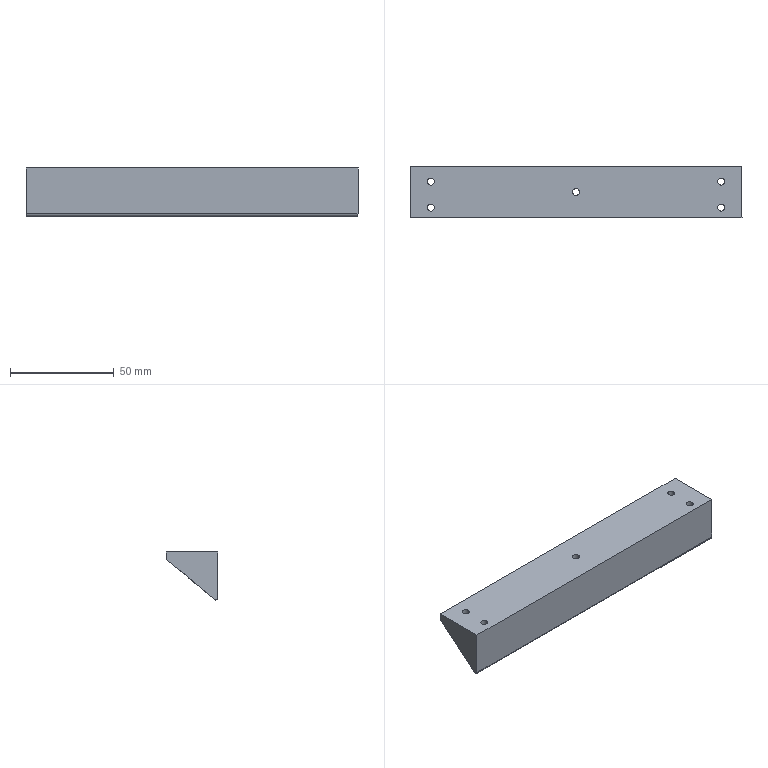Part | SolidWorks | features BaseBody 1, DelFace 1 | 1 solid | 19 faces | box 160 x 25 x 23.134 mm | volume 54327 mm3 | cylinder 13 | plane 6 | commonest cylinder face diameters 3.4 x10 2 x3
STEP:
#1=CARTESIAN_POINT('',(-731.43,686.87,479.692));
#2=VERTEX_POINT('',#1);
#3=CARTESIAN_POINT('',(-734.83,686.87,479.692));
#4=VERTEX_POINT('',#3);
#5=CARTESIAN_POINT('',(-731.43,686.87,479.692));
#6=CARTESIAN_POINT('',(-731.43,690.27,482.545));
#7=CARTESIAN_POINT('',(-734.83,690.27,482.545));
#8=CARTESIAN_POINT('',(-734.83,686.87,479.692));
#9=(BOUNDED_CURVE()B_SPLINE_CURVE(3,(#5,#6,#7,#8),.UNSPECIFIED.,.F.,.F.)B_SPLINE_CURVE_WITH_KNOTS((4,4),(4.712,7.854),.UNSPECIFIED.)CURVE()GEOMETRIC_REPRESENTATION_ITEM()RATIONAL_B_SPLINE_CURVE((1.,0.3333,0.3333,1.))REPRESENTATION_ITEM(''));
#10=EDGE_CURVE('',#2,#4,#9,.T.);
#11=ORIENTED_EDGE('',*,*,#10,.F.);
#12=CARTESIAN_POINT('',(-731.43,686.87,493.482));
#13=VERTEX_POINT('',#12);
#14=CARTESIAN_POINT('',(-731.43,686.87,493.482));
#15=DIRECTION('',(0.,0.,1.));
#16=VECTOR('',#15,1000.);
#17=LINE('',#14,#16);
#18=EDGE_CURVE('',#2,#13,#17,.T.);
#19=ORIENTED_EDGE('',*,*,#18,.T.);
#20=CARTESIAN_POINT('',(-734.83,686.87,493.482));
#21=VERTEX_POINT('',#20);
#22=CARTESIAN_POINT('',(-733.13,686.87,493.482));
#23=DIRECTION('',(0.,0.,1.));
#24=DIRECTION('',(-0.000001544,1.,0.));
#25=AXIS2_PLACEMENT_3D('',#22,#23,#24);
#26=CIRCLE('',#25,1.7);
#27=EDGE_CURVE('',#13,#21,#26,.T.);
#28=ORIENTED_EDGE('',*,*,#27,.T.);
#29=CARTESIAN_POINT('',(-734.83,686.87,493.482));
#30=DIRECTION('',(0.,0.,1.));
#31=VECTOR('',#30,1000.);
#32=LINE('',#29,#31);
#33=EDGE_CURVE('',#4,#21,#32,.T.);
#34=ORIENTED_EDGE('',*,*,#33,.F.);
#35=EDGE_LOOP('',(#11,#19,#28,#34));
#36=FACE_OUTER_BOUND('',#35,.T.);
#37=CARTESIAN_POINT('',(-733.13,686.87,493.482));
#38=DIRECTION('',(0.,0.,1.));
#39=DIRECTION('',(-1.,-0.000001544,0.));
#40=AXIS2_PLACEMENT_3D('',#37,#38,#39);
#41=CYLINDRICAL_SURFACE('',#40,1.7);
#42=ADVANCED_FACE('',(#36),#41,.F.);
#43=CARTESIAN_POINT('',(-661.43,691.87,483.888));
#44=VERTEX_POINT('',#43);
#45=CARTESIAN_POINT('',(-664.83,691.87,483.888));
#46=VERTEX_POINT('',#45);
#47=CARTESIAN_POINT('',(-661.43,691.87,483.888));
#48=CARTESIAN_POINT('',(-661.43,695.27,486.741));
#49=CARTESIAN_POINT('',(-664.83,695.27,486.741));
#50=CARTESIAN_POINT('',(-664.83,691.87,483.888));
#51=(BOUNDED_CURVE()B_SPLINE_CURVE(3,(#47,#48,#49,#50),.UNSPECIFIED.,.F.,.F.)B_SPLINE_CURVE_WITH_KNOTS((4,4),(4.712,7.854),.UNSPECIFIED.)CURVE()GEOMETRIC_REPRESENTATION_ITEM()RATIONAL_B_SPLINE_CURVE((1.,0.3333,0.3333,1.))REPRESENTATION_ITEM(''));
#52=EDGE_CURVE('',#44,#46,#51,.T.);
#53=ORIENTED_EDGE('',*,*,#52,.F.);
#54=CARTESIAN_POINT('',(-661.43,691.87,493.482));
#55=VERTEX_POINT('',#54);
#56=CARTESIAN_POINT('',(-661.43,691.87,493.482));
#57=DIRECTION('',(0.,0.,1.));
#58=VECTOR('',#57,1000.);
#59=LINE('',#56,#58);
#60=EDGE_CURVE('',#44,#55,#59,.T.);
#61=ORIENTED_EDGE('',*,*,#60,.T.);
#62=CARTESIAN_POINT('',(-664.83,691.87,493.482));
#63=VERTEX_POINT('',#62);
#64=CARTESIAN_POINT('',(-663.13,691.87,493.482));
#65=DIRECTION('',(0.,0.,1.));
#66=DIRECTION('',(-0.000001544,1.,0.));
#67=AXIS2_PLACEMENT_3D('',#64,#65,#66);
#68=CIRCLE('',#67,1.7);
#69=EDGE_CURVE('',#55,#63,#68,.T.);
#70=ORIENTED_EDGE('',*,*,#69,.T.);
#71=CARTESIAN_POINT('',(-664.83,691.87,493.482));
#72=DIRECTION('',(0.,0.,1.));
#73=VECTOR('',#72,1000.);
#74=LINE('',#71,#73);
#75=EDGE_CURVE('',#46,#63,#74,.T.);
#76=ORIENTED_EDGE('',*,*,#75,.F.);
#77=EDGE_LOOP('',(#53,#61,#70,#76));
#78=FACE_OUTER_BOUND('',#77,.T.);
#79=CARTESIAN_POINT('',(-663.13,691.87,493.482));
#80=DIRECTION('',(0.,0.,1.));
#81=DIRECTION('',(-1.,-0.000001544,0.));
#82=AXIS2_PLACEMENT_3D('',#79,#80,#81);
#83=CYLINDRICAL_SURFACE('',#82,1.7);
#84=ADVANCED_FACE('',(#78),#83,.F.);
#85=CARTESIAN_POINT('',(-661.43,679.37,473.399));
#86=VERTEX_POINT('',#85);
#87=CARTESIAN_POINT('',(-664.83,679.37,473.399));
#88=VERTEX_POINT('',#87);
#89=CARTESIAN_POINT('',(-661.43,679.37,473.399));
#90=CARTESIAN_POINT('',(-661.43,682.77,476.252));
#91=CARTESIAN_POINT('',(-664.83,682.77,476.252));
#92=CARTESIAN_POINT('',(-664.83,679.37,473.399));
#93=(BOUNDED_CURVE()B_SPLINE_CURVE(3,(#89,#90,#91,#92),.UNSPECIFIED.,.F.,.F.)B_SPLINE_CURVE_WITH_KNOTS((4,4),(4.712,7.854),.UNSPECIFIED.)CURVE()GEOMETRIC_REPRESENTATION_ITEM()RATIONAL_B_SPLINE_CURVE((1.,0.3333,0.3333,1.))REPRESENTATION_ITEM(''));
#94=EDGE_CURVE('',#86,#88,#93,.T.);
#95=ORIENTED_EDGE('',*,*,#94,.F.);
#96=CARTESIAN_POINT('',(-661.43,679.37,493.482));
#97=VERTEX_POINT('',#96);
#98=CARTESIAN_POINT('',(-661.43,679.37,493.482));
#99=DIRECTION('',(0.,0.,1.));
#100=VECTOR('',#99,1000.);
#101=LINE('',#98,#100);
#102=EDGE_CURVE('',#86,#97,#101,.T.);
#103=ORIENTED_EDGE('',*,*,#102,.T.);
#104=CARTESIAN_POINT('',(-664.83,679.37,493.482));
#105=VERTEX_POINT('',#104);
#106=CARTESIAN_POINT('',(-663.13,679.37,493.482));
#107=DIRECTION('',(0.,0.,1.));
#108=DIRECTION('',(-0.000001544,1.,0.));
#109=AXIS2_PLACEMENT_3D('',#106,#107,#108);
#110=CIRCLE('',#109,1.7);
#111=EDGE_CURVE('',#97,#105,#110,.T.);
#112=ORIENTED_EDGE('',*,*,#111,.T.);
#113=CARTESIAN_POINT('',(-664.83,679.37,493.482));
#114=DIRECTION('',(0.,0.,1.));
#115=VECTOR('',#114,1000.);
#116=LINE('',#113,#115);
#117=EDGE_CURVE('',#88,#105,#116,.T.);
#118=ORIENTED_EDGE('',*,*,#117,.F.);
#119=EDGE_LOOP('',(#95,#103,#112,#118));
#120=FACE_OUTER_BOUND('',#119,.T.);
#121=CARTESIAN_POINT('',(-663.13,679.37,493.482));
#122=DIRECTION('',(0.,0.,1.));
#123=DIRECTION('',(-1.,-0.000001544,0.));
#124=AXIS2_PLACEMENT_3D('',#121,#122,#123);
#125=CYLINDRICAL_SURFACE('',#124,1.7);
#126=ADVANCED_FACE('',(#120),#125,.F.);
#127=CARTESIAN_POINT('',(-801.43,691.87,483.888));
#128=VERTEX_POINT('',#127);
#129=CARTESIAN_POINT('',(-804.83,691.87,483.888));
#130=VERTEX_POINT('',#129);
#131=CARTESIAN_POINT('',(-801.43,691.87,483.888));
#132=CARTESIAN_POINT('',(-801.43,695.27,486.741));
#133=CARTESIAN_POINT('',(-804.83,695.27,486.741));
#134=CARTESIAN_POINT('',(-804.83,691.87,483.888));
#135=(BOUNDED_CURVE()B_SPLINE_CURVE(3,(#131,#132,#133,#134),.UNSPECIFIED.,.F.,.F.)B_SPLINE_CURVE_WITH_KNOTS((4,4),(4.712,7.854),.UNSPECIFIED.)CURVE()GEOMETRIC_REPRESENTATION_ITEM()RATIONAL_B_SPLINE_CURVE((1.,0.3333,0.3333,1.))REPRESENTATION_ITEM(''));
#136=EDGE_CURVE('',#128,#130,#135,.T.);
#137=ORIENTED_EDGE('',*,*,#136,.F.);
#138=CARTESIAN_POINT('',(-801.43,691.87,493.482));
#139=VERTEX_POINT('',#138);
#140=CARTESIAN_POINT('',(-801.43,691.87,493.482));
#141=DIRECTION('',(0.,0.,1.));
#142=VECTOR('',#141,1000.);
#143=LINE('',#140,#142);
#144=EDGE_CURVE('',#128,#139,#143,.T.);
#145=ORIENTED_EDGE('',*,*,#144,.T.);
#146=CARTESIAN_POINT('',(-804.83,691.87,493.482));
#147=VERTEX_POINT('',#146);
#148=CARTESIAN_POINT('',(-803.13,691.87,493.482));
#149=DIRECTION('',(0.,0.,1.));
#150=DIRECTION('',(-0.000001544,1.,0.));
#151=AXIS2_PLACEMENT_3D('',#148,#149,#150);
#152=CIRCLE('',#151,1.7);
#153=EDGE_CURVE('',#139,#147,#152,.T.);
#154=ORIENTED_EDGE('',*,*,#153,.T.);
#155=CARTESIAN_POINT('',(-804.83,691.87,493.482));
#156=DIRECTION('',(0.,0.,1.));
#157=VECTOR('',#156,1000.);
#158=LINE('',#155,#157);
#159=EDGE_CURVE('',#130,#147,#158,.T.);
#160=ORIENTED_EDGE('',*,*,#159,.F.);
#161=EDGE_LOOP('',(#137,#145,#154,#160));
#162=FACE_OUTER_BOUND('',#161,.T.);
#163=CARTESIAN_POINT('',(-803.13,691.87,493.482));
#164=DIRECTION('',(0.,0.,1.));
#165=DIRECTION('',(-1.,-0.000001544,0.));
#166=AXIS2_PLACEMENT_3D('',#163,#164,#165);
#167=CYLINDRICAL_SURFACE('',#166,1.7);
#168=ADVANCED_FACE('',(#162),#167,.F.);
#169=CARTESIAN_POINT('',(-801.43,679.37,473.399));
#170=VERTEX_POINT('',#169);
#171=CARTESIAN_POINT('',(-804.83,679.37,473.399));
#172=VERTEX_POINT('',#171);
#173=CARTESIAN_POINT('',(-801.43,679.37,473.399));
#174=CARTESIAN_POINT('',(-801.43,682.77,476.252));
#175=CARTESIAN_POINT('',(-804.83,682.77,476.252));
#176=CARTESIAN_POINT('',(-804.83,679.37,473.399));
#177=(BOUNDED_CURVE()B_SPLINE_CURVE(3,(#173,#174,#175,#176),.UNSPECIFIED.,.F.,.F.)B_SPLINE_CURVE_WITH_KNOTS((4,4),(4.712,7.854),.UNSPECIFIED.)CURVE()GEOMETRIC_REPRESENTATION_ITEM()RATIONAL_B_SPLINE_CURVE((1.,0.3333,0.3333,1.))REPRESENTATION_ITEM(''));
#178=EDGE_CURVE('',#170,#172,#177,.T.);
#179=ORIENTED_EDGE('',*,*,#178,.F.);
#180=CARTESIAN_POINT('',(-801.43,679.37,493.482));
#181=VERTEX_POINT('',#180);
#182=CARTESIAN_POINT('',(-801.43,679.37,493.482));
#183=DIRECTION('',(0.,0.,1.));
#184=VECTOR('',#183,1000.);
#185=LINE('',#182,#184);
#186=EDGE_CURVE('',#170,#181,#185,.T.);
#187=ORIENTED_EDGE('',*,*,#186,.T.);
#188=CARTESIAN_POINT('',(-804.83,679.37,493.482));
#189=VERTEX_POINT('',#188);
#190=CARTESIAN_POINT('',(-803.13,679.37,493.482));
#191=DIRECTION('',(0.,0.,1.));
#192=DIRECTION('',(-0.000001544,1.,0.));
#193=AXIS2_PLACEMENT_3D('',#190,#191,#192);
#194=CIRCLE('',#193,1.7);
#195=EDGE_CURVE('',#181,#189,#194,.T.);
#196=ORIENTED_EDGE('',*,*,#195,.T.);
#197=CARTESIAN_POINT('',(-804.83,679.37,493.482));
#198=DIRECTION('',(0.,0.,1.));
#199=VECTOR('',#198,1000.);
#200=LINE('',#197,#199);
#201=EDGE_CURVE('',#172,#189,#200,.T.);
#202=ORIENTED_EDGE('',*,*,#201,.F.);
#203=EDGE_LOOP('',(#179,#187,#196,#202));
#204=FACE_OUTER_BOUND('',#203,.T.);
#205=CARTESIAN_POINT('',(-803.13,679.37,493.482));
#206=DIRECTION('',(0.,0.,1.));
#207=DIRECTION('',(-1.,-0.000001544,0.));
#208=AXIS2_PLACEMENT_3D('',#205,#206,#207);
#209=CYLINDRICAL_SURFACE('',#208,1.7);
#210=ADVANCED_FACE('',(#204),#209,.F.);
#211=CARTESIAN_POINT('',(-653.13,676.013,470.582));
#212=VERTEX_POINT('',#211);
#213=CARTESIAN_POINT('',(-653.13,675.37,470.348));
#214=VERTEX_POINT('',#213);
#215=CARTESIAN_POINT('',(-653.13,675.37,471.348));
#216=DIRECTION('',(-1.,-0.000001544,0.));
#217=DIRECTION('',(-0.000000993,0.6428,-0.766));
#218=AXIS2_PLACEMENT_3D('',#215,#216,#217);
#219=CIRCLE('',#218,1.);
#220=EDGE_CURVE('',#212,#214,#219,.T.);
#221=ORIENTED_EDGE('',*,*,#220,.T.);
#222=CARTESIAN_POINT('',(-813.13,675.37,470.348));
#223=VERTEX_POINT('',#222);
#224=CARTESIAN_POINT('',(-444.554,675.371,470.348));
#225=DIRECTION('',(-1.,-0.000001544,0.));
#226=VECTOR('',#225,1000.);
#227=LINE('',#224,#226);
#228=EDGE_CURVE('',#214,#223,#227,.T.);
#229=ORIENTED_EDGE('',*,*,#228,.T.);
#230=CARTESIAN_POINT('',(-813.13,676.013,470.582));
#231=VERTEX_POINT('',#230);
#232=CARTESIAN_POINT('',(-813.13,675.37,471.348));
#233=DIRECTION('',(1.,0.000001544,0.));
#234=DIRECTION('',(0.000001544,-1.,0.));
#235=AXIS2_PLACEMENT_3D('',#232,#233,#234);
#236=CIRCLE('',#235,1.);
#237=EDGE_CURVE('',#223,#231,#236,.T.);
#238=ORIENTED_EDGE('',*,*,#237,.T.);
#239=CARTESIAN_POINT('',(-653.13,676.013,470.582));
#240=DIRECTION('',(-1.,-0.000001544,0.));
#241=VECTOR('',#240,1000.);
#242=LINE('',#239,#241);
#243=EDGE_CURVE('',#212,#231,#242,.T.);
#244=ORIENTED_EDGE('',*,*,#243,.F.);
#245=EDGE_LOOP('',(#221,#229,#238,#244));
#246=FACE_OUTER_BOUND('',#245,.T.);
#247=CARTESIAN_POINT('',(-444.554,675.371,471.348));
#248=DIRECTION('',(-1.,-0.000001544,0.));
#249=DIRECTION('',(0.,0.,-1.));
#250=AXIS2_PLACEMENT_3D('',#247,#248,#249);
#251=CYLINDRICAL_SURFACE('',#250,1.);
#252=ADVANCED_FACE('',(#246),#251,.T.);
#253=CARTESIAN_POINT('',(-653.13,674.37,493.482));
#254=VERTEX_POINT('',#253);
#255=CARTESIAN_POINT('',(-653.13,699.37,493.482));
#256=VERTEX_POINT('',#255);
#257=CARTESIAN_POINT('',(-653.13,674.37,493.482));
#258=DIRECTION('',(-0.000001544,1.,0.));
#259=VECTOR('',#258,1000.);
#260=LINE('',#257,#259);
#261=EDGE_CURVE('',#254,#256,#260,.T.);
#262=ORIENTED_EDGE('',*,*,#261,.F.);
#263=CARTESIAN_POINT('',(-653.13,674.37,471.348));
#264=VERTEX_POINT('',#263);
#265=CARTESIAN_POINT('',(-653.13,674.37,471.348));
#266=DIRECTION('',(0.,0.,1.));
#267=VECTOR('',#266,1000.);
#268=LINE('',#265,#267);
#269=EDGE_CURVE('',#264,#254,#268,.T.);
#270=ORIENTED_EDGE('',*,*,#269,.F.);
#271=CARTESIAN_POINT('',(-653.13,675.37,471.348));
#272=DIRECTION('',(-1.,-0.000001544,0.));
#273=DIRECTION('',(-0.000000993,0.6428,-0.766));
#274=AXIS2_PLACEMENT_3D('',#271,#272,#273);
#275=CIRCLE('',#274,1.);
#276=EDGE_CURVE('',#214,#264,#275,.T.);
#277=ORIENTED_EDGE('',*,*,#276,.F.);
#278=ORIENTED_EDGE('',*,*,#220,.F.);
#279=CARTESIAN_POINT('',(-653.13,699.013,489.881));
#280=VERTEX_POINT('',#279);
#281=CARTESIAN_POINT('',(-653.13,699.013,489.881));
#282=DIRECTION('',(0.000001183,-0.766,-0.6428));
#283=VECTOR('',#282,1000.);
#284=LINE('',#281,#283);
#285=EDGE_CURVE('',#280,#212,#284,.T.);
#286=ORIENTED_EDGE('',*,*,#285,.F.);
#287=CARTESIAN_POINT('',(-653.13,699.37,490.647));
#288=VERTEX_POINT('',#287);
#289=CARTESIAN_POINT('',(-653.13,698.37,490.647));
#290=DIRECTION('',(-1.,-0.000001544,0.));
#291=DIRECTION('',(-0.000001544,1.,0.));
#292=AXIS2_PLACEMENT_3D('',#289,#290,#291);
#293=CIRCLE('',#292,1.);
#294=EDGE_CURVE('',#288,#280,#293,.T.);
#295=ORIENTED_EDGE('',*,*,#294,.F.);
#296=CARTESIAN_POINT('',(-653.13,699.37,493.482));
#297=DIRECTION('',(0.,0.,-1.));
#298=VECTOR('',#297,1000.);
#299=LINE('',#296,#298);
#300=EDGE_CURVE('',#256,#288,#299,.T.);
#301=ORIENTED_EDGE('',*,*,#300,.F.);
#302=EDGE_LOOP('',(#262,#270,#277,#278,#286,#295,#301));
#303=FACE_OUTER_BOUND('',#302,.T.);
#304=CARTESIAN_POINT('',(-653.129,0.00034,130.75));
#305=DIRECTION('',(1.,0.000001544,0.));
#306=DIRECTION('',(0.000001544,-1.,0.));
#307=AXIS2_PLACEMENT_3D('',#304,#305,#306);
#308=PLANE('',#307);
#309=ADVANCED_FACE('',(#303),#308,.T.);
#310=CARTESIAN_POINT('',(-813.13,699.37,493.482));
#311=VERTEX_POINT('',#310);
#312=CARTESIAN_POINT('',(-653.13,699.37,493.482));
#313=DIRECTION('',(-1.,-0.000001544,0.));
#314=VECTOR('',#313,1000.);
#315=LINE('',#312,#314);
#316=EDGE_CURVE('',#256,#311,#315,.T.);
#317=ORIENTED_EDGE('',*,*,#316,.F.);
#318=ORIENTED_EDGE('',*,*,#300,.T.);
#319=CARTESIAN_POINT('',(-813.13,699.37,490.647));
#320=VERTEX_POINT('',#319);
#321=CARTESIAN_POINT('',(-653.13,699.37,490.647));
#322=DIRECTION('',(-1.,-0.000001544,0.));
#323=VECTOR('',#322,1000.);
#324=LINE('',#321,#323);
#325=EDGE_CURVE('',#288,#320,#324,.T.);
#326=ORIENTED_EDGE('',*,*,#325,.T.);
#327=CARTESIAN_POINT('',(-813.13,699.37,490.647));
#328=DIRECTION('',(0.,0.,1.));
#329=VECTOR('',#328,1000.);
#330=LINE('',#327,#329);
#331=EDGE_CURVE('',#320,#311,#330,.T.);
#332=ORIENTED_EDGE('',*,*,#331,.T.);
#333=EDGE_LOOP('',(#317,#318,#326,#332));
#334=FACE_OUTER_BOUND('',#333,.T.);
#335=CARTESIAN_POINT('',(-653.13,699.37,490.349));
#336=DIRECTION('',(-0.000001544,1.,0.));
#337=DIRECTION('',(0.,0.,-1.));
#338=AXIS2_PLACEMENT_3D('',#335,#336,#337);
#339=PLANE('',#338);
#340=ADVANCED_FACE('',(#334),#339,.T.);
#341=CARTESIAN_POINT('',(-813.13,699.013,489.881));
#342=VERTEX_POINT('',#341);
#343=CARTESIAN_POINT('',(-813.13,676.013,470.582));
#344=DIRECTION('',(-0.000001183,0.766,0.6428));
#345=VECTOR('',#344,1000.);
#346=LINE('',#343,#345);
#347=EDGE_CURVE('',#231,#342,#346,.T.);
#348=ORIENTED_EDGE('',*,*,#347,.F.);
#349=ORIENTED_EDGE('',*,*,#237,.F.);
#350=CARTESIAN_POINT('',(-813.13,674.37,471.348));
#351=VERTEX_POINT('',#350);
#352=CARTESIAN_POINT('',(-813.13,675.37,471.348));
#353=DIRECTION('',(1.,0.000001544,0.));
#354=DIRECTION('',(0.000001544,-1.,0.));
#355=AXIS2_PLACEMENT_3D('',#352,#353,#354);
#356=CIRCLE('',#355,1.);
#357=EDGE_CURVE('',#351,#223,#356,.T.);
#358=ORIENTED_EDGE('',*,*,#357,.F.);
#359=CARTESIAN_POINT('',(-813.13,674.37,493.482));
#360=VERTEX_POINT('',#359);
#361=CARTESIAN_POINT('',(-813.13,674.37,493.482));
#362=DIRECTION('',(0.,0.,-1.));
#363=VECTOR('',#362,1000.);
#364=LINE('',#361,#363);
#365=EDGE_CURVE('',#360,#351,#364,.T.);
#366=ORIENTED_EDGE('',*,*,#365,.F.);
#367=CARTESIAN_POINT('',(-813.13,699.37,493.482));
#368=DIRECTION('',(0.000001544,-1.,0.));
#369=VECTOR('',#368,1000.);
#370=LINE('',#367,#369);
#371=EDGE_CURVE('',#311,#360,#370,.T.);
#372=ORIENTED_EDGE('',*,*,#371,.F.);
#373=ORIENTED_EDGE('',*,*,#331,.F.);
#374=CARTESIAN_POINT('',(-813.13,698.37,490.647));
#375=DIRECTION('',(1.,0.000001544,0.));
#376=DIRECTION('',(-0.000000993,0.6428,-0.766));
#377=AXIS2_PLACEMENT_3D('',#374,#375,#376);
#378=CIRCLE('',#377,1.);
#379=EDGE_CURVE('',#342,#320,#378,.T.);
#380=ORIENTED_EDGE('',*,*,#379,.F.);
#381=EDGE_LOOP('',(#348,#349,#358,#366,#372,#373,#380));
#382=FACE_OUTER_BOUND('',#381,.T.);
#383=CARTESIAN_POINT('',(-813.13,738.297,503.482));
#384=DIRECTION('',(-1.,-0.000001544,0.));
#385=DIRECTION('',(-0.000001544,1.,0.));
#386=AXIS2_PLACEMENT_3D('',#383,#384,#385);
#387=PLANE('',#386);
#388=ADVANCED_FACE('',(#382),#387,.T.);
#389=ORIENTED_EDGE('',*,*,#243,.T.);
#390=ORIENTED_EDGE('',*,*,#347,.T.);
#391=CARTESIAN_POINT('',(-813.13,699.013,489.881));
#392=DIRECTION('',(1.,0.000001544,0.));
#393=VECTOR('',#392,1000.);
#394=LINE('',#391,#393);
#395=EDGE_CURVE('',#342,#280,#394,.T.);
#396=ORIENTED_EDGE('',*,*,#395,.T.);
#397=ORIENTED_EDGE('',*,*,#285,.T.);
#398=EDGE_LOOP('',(#389,#390,#396,#397));
#399=FACE_OUTER_BOUND('',#398,.T.);
#400=CARTESIAN_POINT('',(-804.83,679.37,473.399));
#401=CARTESIAN_POINT('',(-804.83,675.97,470.546));
#402=CARTESIAN_POINT('',(-801.43,675.97,470.546));
#403=CARTESIAN_POINT('',(-801.43,679.37,473.399));
#404=(BOUNDED_CURVE()B_SPLINE_CURVE(3,(#400,#401,#402,#403),.UNSPECIFIED.,.F.,.F.)B_SPLINE_CURVE_WITH_KNOTS((4,4),(1.571,4.712),.UNSPECIFIED.)CURVE()GEOMETRIC_REPRESENTATION_ITEM()RATIONAL_B_SPLINE_CURVE((1.,0.3333,0.3333,1.))REPRESENTATION_ITEM(''));
#405=EDGE_CURVE('',#172,#170,#404,.T.);
#406=ORIENTED_EDGE('',*,*,#405,.T.);
#407=ORIENTED_EDGE('',*,*,#178,.T.);
#408=EDGE_LOOP('',(#406,#407));
#409=FACE_BOUND('',#408,.T.);
#410=CARTESIAN_POINT('',(-664.83,691.87,483.888));
#411=CARTESIAN_POINT('',(-664.83,688.47,481.035));
#412=CARTESIAN_POINT('',(-661.43,688.47,481.035));
#413=CARTESIAN_POINT('',(-661.43,691.87,483.888));
#414=(BOUNDED_CURVE()B_SPLINE_CURVE(3,(#410,#411,#412,#413),.UNSPECIFIED.,.F.,.F.)B_SPLINE_CURVE_WITH_KNOTS((4,4),(1.571,4.712),.UNSPECIFIED.)CURVE()GEOMETRIC_REPRESENTATION_ITEM()RATIONAL_B_SPLINE_CURVE((1.,0.3333,0.3333,1.))REPRESENTATION_ITEM(''));
#415=EDGE_CURVE('',#46,#44,#414,.T.);
#416=ORIENTED_EDGE('',*,*,#415,.T.);
#417=ORIENTED_EDGE('',*,*,#52,.T.);
#418=EDGE_LOOP('',(#416,#417));
#419=FACE_BOUND('',#418,.T.);
#420=CARTESIAN_POINT('',(-664.83,679.37,473.399));
#421=CARTESIAN_POINT('',(-664.83,675.97,470.546));
#422=CARTESIAN_POINT('',(-661.43,675.97,470.546));
#423=CARTESIAN_POINT('',(-661.43,679.37,473.399));
#424=(BOUNDED_CURVE()B_SPLINE_CURVE(3,(#420,#421,#422,#423),.UNSPECIFIED.,.F.,.F.)B_SPLINE_CURVE_WITH_KNOTS((4,4),(1.571,4.712),.UNSPECIFIED.)CURVE()GEOMETRIC_REPRESENTATION_ITEM()RATIONAL_B_SPLINE_CURVE((1.,0.3333,0.3333,1.))REPRESENTATION_ITEM(''));
#425=EDGE_CURVE('',#88,#86,#424,.T.);
#426=ORIENTED_EDGE('',*,*,#425,.T.);
#427=ORIENTED_EDGE('',*,*,#94,.T.);
#428=EDGE_LOOP('',(#426,#427));
#429=FACE_BOUND('',#428,.T.);
#430=CARTESIAN_POINT('',(-734.83,686.87,479.692));
#431=CARTESIAN_POINT('',(-734.83,683.47,476.839));
#432=CARTESIAN_POINT('',(-731.43,683.47,476.839));
#433=CARTESIAN_POINT('',(-731.43,686.87,479.692));
#434=(BOUNDED_CURVE()B_SPLINE_CURVE(3,(#430,#431,#432,#433),.UNSPECIFIED.,.F.,.F.)B_SPLINE_CURVE_WITH_KNOTS((4,4),(1.571,4.712),.UNSPECIFIED.)CURVE()GEOMETRIC_REPRESENTATION_ITEM()RATIONAL_B_SPLINE_CURVE((1.,0.3333,0.3333,1.))REPRESENTATION_ITEM(''));
#435=EDGE_CURVE('',#4,#2,#434,.T.);
#436=ORIENTED_EDGE('',*,*,#435,.T.);
#437=ORIENTED_EDGE('',*,*,#10,.T.);
#438=EDGE_LOOP('',(#436,#437));
#439=FACE_BOUND('',#438,.T.);
#440=CARTESIAN_POINT('',(-804.83,691.87,483.888));
#441=CARTESIAN_POINT('',(-804.83,688.47,481.035));
#442=CARTESIAN_POINT('',(-801.43,688.47,481.035));
#443=CARTESIAN_POINT('',(-801.43,691.87,483.888));
#444=(BOUNDED_CURVE()B_SPLINE_CURVE(3,(#440,#441,#442,#443),.UNSPECIFIED.,.F.,.F.)B_SPLINE_CURVE_WITH_KNOTS((4,4),(1.571,4.712),.UNSPECIFIED.)CURVE()GEOMETRIC_REPRESENTATION_ITEM()RATIONAL_B_SPLINE_CURVE((1.,0.3333,0.3333,1.))REPRESENTATION_ITEM(''));
#445=EDGE_CURVE('',#130,#128,#444,.T.);
#446=ORIENTED_EDGE('',*,*,#445,.T.);
#447=ORIENTED_EDGE('',*,*,#136,.T.);
#448=EDGE_LOOP('',(#446,#447));
#449=FACE_BOUND('',#448,.T.);
#450=CARTESIAN_POINT('',(-653.13,674.37,469.204));
#451=DIRECTION('',(-0.000000993,0.6428,-0.766));
#452=DIRECTION('',(0.000001183,-0.766,-0.6428));
#453=AXIS2_PLACEMENT_3D('',#450,#451,#452);
#454=PLANE('',#453);
#455=ADVANCED_FACE('',(#399,#409,#419,#429,#439,#449),#454,.T.);
#456=ORIENTED_EDGE('',*,*,#294,.T.);
#457=ORIENTED_EDGE('',*,*,#395,.F.);
#458=ORIENTED_EDGE('',*,*,#379,.T.);
#459=ORIENTED_EDGE('',*,*,#325,.F.);
#460=EDGE_LOOP('',(#456,#457,#458,#459));
#461=FACE_OUTER_BOUND('',#460,.T.);
#462=CARTESIAN_POINT('',(-444.554,698.371,490.647));
#463=DIRECTION('',(-1.,-0.000001544,0.));
#464=DIRECTION('',(0.,0.,-1.));
#465=AXIS2_PLACEMENT_3D('',#462,#463,#464);
#466=CYLINDRICAL_SURFACE('',#465,1.);
#467=ADVANCED_FACE('',(#461),#466,.T.);
#468=ORIENTED_EDGE('',*,*,#228,.F.);
#469=ORIENTED_EDGE('',*,*,#276,.T.);
#470=CARTESIAN_POINT('',(-813.13,674.37,471.348));
#471=DIRECTION('',(1.,0.000001544,0.));
#472=VECTOR('',#471,1000.);
#473=LINE('',#470,#472);
#474=EDGE_CURVE('',#351,#264,#473,.T.);
#475=ORIENTED_EDGE('',*,*,#474,.F.);
#476=ORIENTED_EDGE('',*,*,#357,.T.);
#477=EDGE_LOOP('',(#468,#469,#475,#476));
#478=FACE_OUTER_BOUND('',#477,.T.);
#479=CARTESIAN_POINT('',(-444.554,675.371,471.348));
#480=DIRECTION('',(-1.,-0.000001544,0.));
#481=DIRECTION('',(0.,0.,-1.));
#482=AXIS2_PLACEMENT_3D('',#479,#480,#481);
#483=CYLINDRICAL_SURFACE('',#482,1.);
#484=ADVANCED_FACE('',(#478),#483,.T.);
#485=CARTESIAN_POINT('',(-653.13,674.37,493.482));
#486=DIRECTION('',(-1.,-0.000001544,0.));
#487=VECTOR('',#486,1000.);
#488=LINE('',#485,#487);
#489=EDGE_CURVE('',#254,#360,#488,.T.);
#490=ORIENTED_EDGE('',*,*,#489,.T.);
#491=ORIENTED_EDGE('',*,*,#365,.T.);
#492=ORIENTED_EDGE('',*,*,#474,.T.);
#493=ORIENTED_EDGE('',*,*,#269,.T.);
#494=EDGE_LOOP('',(#490,#491,#492,#493));
#495=FACE_OUTER_BOUND('',#494,.T.);
#496=CARTESIAN_POINT('',(-653.13,674.37,493.482));
#497=DIRECTION('',(0.000001544,-1.,0.));
#498=DIRECTION('',(0.,0.,1.));
#499=AXIS2_PLACEMENT_3D('',#496,#497,#498);
#500=PLANE('',#499);
#501=ADVANCED_FACE('',(#495),#500,.T.);
#502=ORIENTED_EDGE('',*,*,#371,.T.);
#503=ORIENTED_EDGE('',*,*,#489,.F.);
#504=ORIENTED_EDGE('',*,*,#261,.T.);
#505=ORIENTED_EDGE('',*,*,#316,.T.);
#506=EDGE_LOOP('',(#502,#503,#504,#505));
#507=FACE_OUTER_BOUND('',#506,.T.);
#508=CARTESIAN_POINT('',(-803.13,679.37,493.482));
#509=DIRECTION('',(0.,0.,1.));
#510=DIRECTION('',(-0.000001544,1.,0.));
#511=AXIS2_PLACEMENT_3D('',#508,#509,#510);
#512=CIRCLE('',#511,1.7);
#513=EDGE_CURVE('',#189,#181,#512,.T.);
#514=ORIENTED_EDGE('',*,*,#513,.F.);
#515=ORIENTED_EDGE('',*,*,#195,.F.);
#516=EDGE_LOOP('',(#514,#515));
#517=FACE_BOUND('',#516,.T.);
#518=CARTESIAN_POINT('',(-803.13,691.87,493.482));
#519=DIRECTION('',(0.,0.,1.));
#520=DIRECTION('',(-0.000001544,1.,0.));
#521=AXIS2_PLACEMENT_3D('',#518,#519,#520);
#522=CIRCLE('',#521,1.7);
#523=EDGE_CURVE('',#147,#139,#522,.T.);
#524=ORIENTED_EDGE('',*,*,#523,.F.);
#525=ORIENTED_EDGE('',*,*,#153,.F.);
#526=EDGE_LOOP('',(#524,#525));
#527=FACE_BOUND('',#526,.T.);
#528=CARTESIAN_POINT('',(-663.13,679.37,493.482));
#529=DIRECTION('',(0.,0.,1.));
#530=DIRECTION('',(-0.000001544,1.,0.));
#531=AXIS2_PLACEMENT_3D('',#528,#529,#530);
#532=CIRCLE('',#531,1.7);
#533=EDGE_CURVE('',#105,#97,#532,.T.);
#534=ORIENTED_EDGE('',*,*,#533,.F.);
#535=ORIENTED_EDGE('',*,*,#111,.F.);
#536=EDGE_LOOP('',(#534,#535));
#537=FACE_BOUND('',#536,.T.);
#538=CARTESIAN_POINT('',(-663.13,691.87,493.482));
#539=DIRECTION('',(0.,0.,1.));
#540=DIRECTION('',(-0.000001544,1.,0.));
#541=AXIS2_PLACEMENT_3D('',#538,#539,#540);
#542=CIRCLE('',#541,1.7);
#543=EDGE_CURVE('',#63,#55,#542,.T.);
#544=ORIENTED_EDGE('',*,*,#543,.F.);
#545=ORIENTED_EDGE('',*,*,#69,.F.);
#546=EDGE_LOOP('',(#544,#545));
#547=FACE_BOUND('',#546,.T.);
#548=CARTESIAN_POINT('',(-733.13,686.87,493.482));
#549=DIRECTION('',(0.,0.,1.));
#550=DIRECTION('',(-0.000001544,1.,0.));
#551=AXIS2_PLACEMENT_3D('',#548,#549,#550);
#552=CIRCLE('',#551,1.7);
#553=EDGE_CURVE('',#21,#13,#552,.T.);
#554=ORIENTED_EDGE('',*,*,#553,.F.);
#555=ORIENTED_EDGE('',*,*,#27,.F.);
#556=EDGE_LOOP('',(#554,#555));
#557=FACE_BOUND('',#556,.T.);
#558=CARTESIAN_POINT('',(-653.13,699.37,493.482));
#559=DIRECTION('',(0.,0.,1.));
#560=DIRECTION('',(-0.000001544,1.,0.));
#561=AXIS2_PLACEMENT_3D('',#558,#559,#560);
#562=PLANE('',#561);
#563=ADVANCED_FACE('',(#507,#517,#527,#537,#547,#557),#562,.T.);
#564=ORIENTED_EDGE('',*,*,#186,.F.);
#565=ORIENTED_EDGE('',*,*,#405,.F.);
#566=ORIENTED_EDGE('',*,*,#201,.T.);
#567=ORIENTED_EDGE('',*,*,#513,.T.);
#568=EDGE_LOOP('',(#564,#565,#566,#567));
#569=FACE_OUTER_BOUND('',#568,.T.);
#570=CARTESIAN_POINT('',(-803.13,679.37,493.482));
#571=DIRECTION('',(0.,0.,1.));
#572=DIRECTION('',(-1.,-0.000001544,0.));
#573=AXIS2_PLACEMENT_3D('',#570,#571,#572);
#574=CYLINDRICAL_SURFACE('',#573,1.7);
#575=ADVANCED_FACE('',(#569),#574,.F.);
#576=ORIENTED_EDGE('',*,*,#144,.F.);
#577=ORIENTED_EDGE('',*,*,#445,.F.);
#578=ORIENTED_EDGE('',*,*,#159,.T.);
#579=ORIENTED_EDGE('',*,*,#523,.T.);
#580=EDGE_LOOP('',(#576,#577,#578,#579));
#581=FACE_OUTER_BOUND('',#580,.T.);
#582=CARTESIAN_POINT('',(-803.13,691.87,493.482));
#583=DIRECTION('',(0.,0.,1.));
#584=DIRECTION('',(-1.,-0.000001544,0.));
#585=AXIS2_PLACEMENT_3D('',#582,#583,#584);
#586=CYLINDRICAL_SURFACE('',#585,1.7);
#587=ADVANCED_FACE('',(#581),#586,.F.);
#588=ORIENTED_EDGE('',*,*,#102,.F.);
#589=ORIENTED_EDGE('',*,*,#425,.F.);
#590=ORIENTED_EDGE('',*,*,#117,.T.);
#591=ORIENTED_EDGE('',*,*,#533,.T.);
#592=EDGE_LOOP('',(#588,#589,#590,#591));
#593=FACE_OUTER_BOUND('',#592,.T.);
#594=CARTESIAN_POINT('',(-663.13,679.37,493.482));
#595=DIRECTION('',(0.,0.,1.));
#596=DIRECTION('',(-1.,-0.000001544,0.));
#597=AXIS2_PLACEMENT_3D('',#594,#595,#596);
#598=CYLINDRICAL_SURFACE('',#597,1.7);
#599=ADVANCED_FACE('',(#593),#598,.F.);
#600=ORIENTED_EDGE('',*,*,#60,.F.);
#601=ORIENTED_EDGE('',*,*,#415,.F.);
#602=ORIENTED_EDGE('',*,*,#75,.T.);
#603=ORIENTED_EDGE('',*,*,#543,.T.);
#604=EDGE_LOOP('',(#600,#601,#602,#603));
#605=FACE_OUTER_BOUND('',#604,.T.);
#606=CARTESIAN_POINT('',(-663.13,691.87,493.482));
#607=DIRECTION('',(0.,0.,1.));
#608=DIRECTION('',(-1.,-0.000001544,0.));
#609=AXIS2_PLACEMENT_3D('',#606,#607,#608);
#610=CYLINDRICAL_SURFACE('',#609,1.7);
#611=ADVANCED_FACE('',(#605),#610,.F.);
#612=ORIENTED_EDGE('',*,*,#18,.F.);
#613=ORIENTED_EDGE('',*,*,#435,.F.);
#614=ORIENTED_EDGE('',*,*,#33,.T.);
#615=ORIENTED_EDGE('',*,*,#553,.T.);
#616=EDGE_LOOP('',(#612,#613,#614,#615));
#617=FACE_OUTER_BOUND('',#616,.T.);
#618=CARTESIAN_POINT('',(-733.13,686.87,493.482));
#619=DIRECTION('',(0.,0.,1.));
#620=DIRECTION('',(-1.,-0.000001544,0.));
#621=AXIS2_PLACEMENT_3D('',#618,#619,#620);
#622=CYLINDRICAL_SURFACE('',#621,1.7);
#623=ADVANCED_FACE('',(#617),#622,.F.);
#624=CLOSED_SHELL('',(#42,#84,#126,#168,#210,#252,#309,#340,#388,#455,#467,#484,#501,#563,#575,#587,#599,#611,#623));
#625=MANIFOLD_SOLID_BREP('',#624);
#626=CARTESIAN_POINT('',(0.,0.,0.));
#627=DIRECTION('',(0.,0.,1.));
#628=DIRECTION('',(1.,0.,0.));
#629=AXIS2_PLACEMENT_3D('',#626,#627,#628);
#630=(LENGTH_UNIT()NAMED_UNIT(*)SI_UNIT(.MILLI.,.METRE.));
#631=UNCERTAINTY_MEASURE_WITH_UNIT(LENGTH_MEASURE(0.00001),#630,'','');
#632=(NAMED_UNIT(*)PLANE_ANGLE_UNIT()SI_UNIT($,.RADIAN.));
#633=(NAMED_UNIT(*)SI_UNIT($,.STERADIAN.)SOLID_ANGLE_UNIT());
#634=(GEOMETRIC_REPRESENTATION_CONTEXT(3)GLOBAL_UNCERTAINTY_ASSIGNED_CONTEXT((#631))GLOBAL_UNIT_ASSIGNED_CONTEXT((#630,#632,#633))REPRESENTATION_CONTEXT('',''));
#635=ADVANCED_BREP_SHAPE_REPRESENTATION('',(#625,#629),#634);